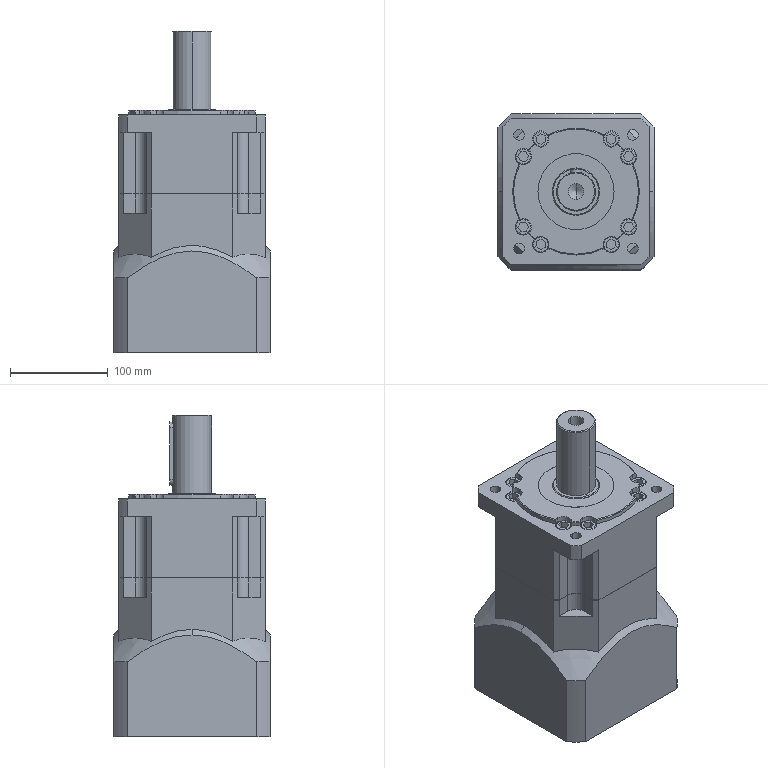Part | SolidWorks | features ICE 18, CirPattern 4, Fillet 2, Revolution 2, Chamfer 1, RevCut 1 | 2 solids | 330 faces | box 160 x 160 x 330 mm | volume 5402193 mm3 | plane 179 | cylinder 110 | torus 24 | cone 17 | commonest cylinder face diameters 16.5 x16 16.8 x16 12 x11 130 x9 8 x8 11 x8